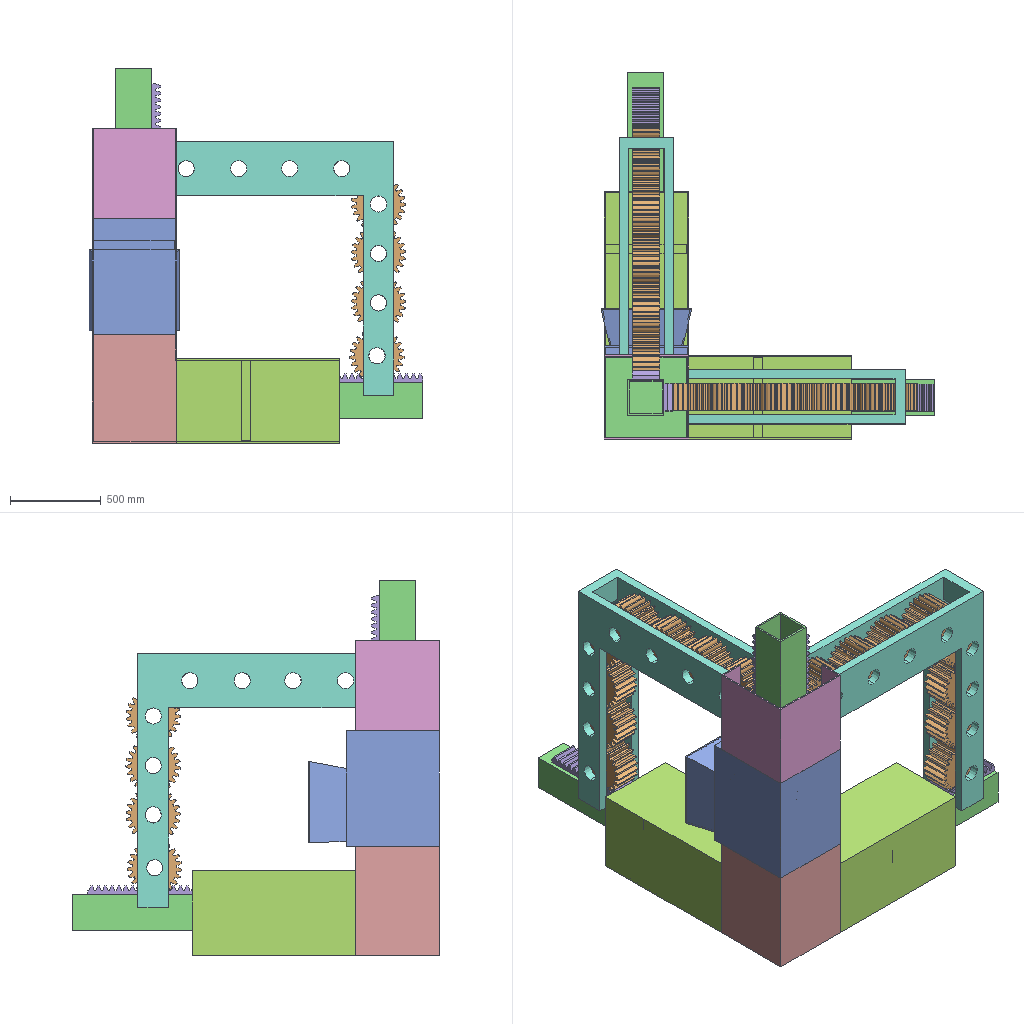Assembly | SolidWorks | 8 different items | 30 placed | box 1844 x 2026 x 2068 mm
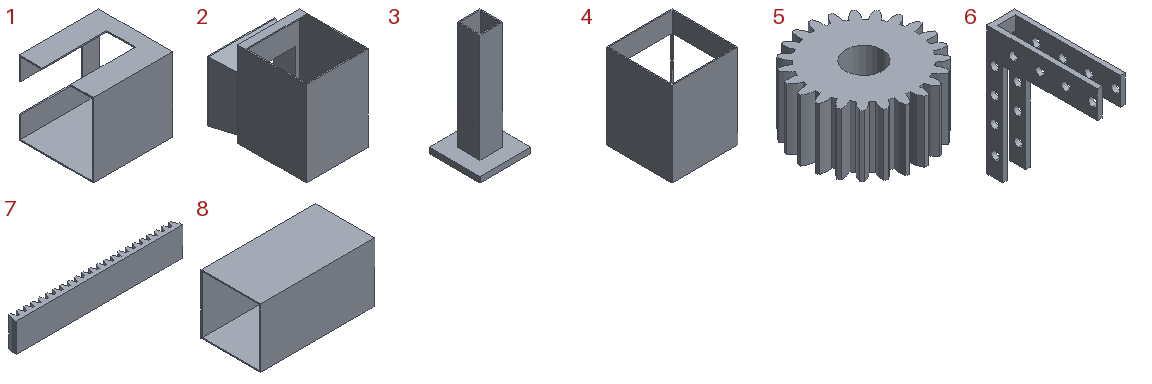Parts list (item | quantity | size | volume | features):
1 | x1 | 500 x 466 x 466 mm | 6178880 mm3 | features Cut 2, DeleteBody 1, Extrusion 1, MoveCopyBody 1, Stock 1
2 | x1 | 500 x 724 x 640 mm | 11993841 mm3 | features ICE 5, Blend 1, Extrusion 1, Shell 1
3 | x3 | 445 x 445 x 1000 mm | 17121250 mm3 | features Extrusion 1, ICE 1
4 | x1 | 466 x 466 x 600 mm | 7173600 mm3 | features ICE 3, Extrusion 1
5 | x16 | 299.728 x 299.348 x 150 mm | 7864200 mm3 | features ICE 2, CirPattern 1, Extrusion 1
6 | x2 | 300 x 1200 x 1400 mm | 51410620 mm3 | features ICE 6, Cut 3, Extrusion 1
7 | x4 | 867.08 x 47 x 150 mm | 4458786 mm3 | features Extrusion 1, ICE 1
8 | x2 | 900 x 466 x 466 mm | 13190400 mm3 | features Extrusion 1
Mates (type | each side: item.copy, entity, surface, feature):
Coincident | 4.1 face plane Boss-Extrude1 | 2.1 face plane Boss-Extrude1 | 3 times
Coincident | 4.1 face plane Boss-Extrude1 | 8.1 face plane Boss-Extrude1 | 3 times
Coincident | 2.1 face plane Boss-Extrude1 | 1.1 face plane Boss-Extrude1 | 3 times
Coincident | 4.1 face plane Boss-Extrude1 | 8.2 face plane Boss-Extrude1 | 3 times
DistanceDim | assembly face | 1.1 face plane Boss-Extrude1 | 2 times
DistanceDim | assembly face | 8.1 face plane Boss-Extrude1
DistanceDim | 8.1 face plane Boss-Extrude1 | assembly face
DistanceDim | assembly face | 8.2 face plane Boss-Extrude1
DistanceDim | 8.2 face plane Boss-Extrude1 | assembly face
DistanceDim | assembly face | 4.1 face plane Boss-Extrude2
DistanceDim | assembly face | 4.1 face plane Boss-Extrude1
DistanceDim | 4.1 face plane Boss-Extrude1 | assembly face
Coincident | 1.1 face plane Boss-Extrude1 | 6.1 face plane Boss-Extrude1
Width | 8.2 face plane Boss-Extrude1 | 8.2 face plane Boss-Extrude1 | 6.1 face plane Boss-Extrude1 | 6.1 face plane Boss-Extrude1
Coincident | 1.1 face plane Boss-Extrude1 | 6.2 face plane Boss-Extrude1
Width | 8.1 face plane Boss-Extrude1 | 8.1 face plane Boss-Extrude1 | 6.2 face plane Boss-Extrude1 | 6.2 face plane Boss-Extrude1
Concentric | 6.1 face cylinder Cut-Extrude2 | 5.1 face cylinder Cut-Extrude1
Width | 6.1 face plane Boss-Extrude1 | 6.1 face plane Boss-Extrude1 | 5.1 face plane Boss-Extrude1 | 5.1 face plane Boss-Extrude1
Parallel | 6.1 face plane Boss-Extrude1 | assembly face | 2 times
Width | 6.1 face plane Boss-Extrude1 | 6.1 face plane Boss-Extrude1 | assembly face | assembly face | 2 times
Coincident | assembly face | 7.1 face plane Boss-Extrude1 | 2 times
Width | assembly face | assembly face | 7.1 face plane Boss-Extrude1 | 7.1 face plane Boss-Extrude1
Concentric | 6.1 face cylinder Cut-Extrude2 | 5.2 face cylinder Cut-Extrude1
Coincident | 5.1 face plane Boss-Extrude1 | 5.2 face plane Boss-Extrude1
Coincident | 8.2 face plane Boss-Extrude1 | assembly face
Coincident | 5.2 face plane Boss-Extrude1 | assembly face
Concentric | 6.1 face cylinder Cut-Extrude2 | 5.3 face cylinder Cut-Extrude1
Concentric | 6.1 face cylinder Cut-Extrude1 | 5.4 face cylinder Cut-Extrude1
Coincident | 5.3 face plane Boss-Extrude1 | 5.4 face plane Boss-Extrude1
Parallel | 5.1 face plane Boss-Extrude1 | 5.3 face plane Boss-Extrude1
Coincident | 5.1 face plane Boss-Extrude1 | 5.3 face plane Boss-Extrude1
GearDim | 5.4 face cylinder Boss-Extrude1 | 5.3 face cylinder CirPattern1
GearDim | 5.1 face cylinder Boss-Extrude2 | 5.3 face cylinder Boss-Extrude1
GearDim | 5.1 face cylinder Boss-Extrude1 | 5.2 face cylinder CirPattern1
Coincident | 5.2 face plane Boss-Extrude1 | 5.5 face plane Boss-Extrude1
Concentric | 6.1 face cylinder Cut-Extrude4 | 5.5 face cylinder Cut-Extrude1
Coincident | 8.2 face plane Boss-Extrude1 | 3.1 face plane Boss-Extrude1 | 2 times
Width | 3.1 face plane Boss-Extrude2 | 3.1 face plane Boss-Extrude2 | 7.1 face plane Boss-Extrude1 | 7.1 face plane Boss-Extrude1
Coincident | 7.1 face plane Boss-Extrude1 | 3.1 face plane Boss-Extrude2
Coincident | 7.1 face plane Boss-Extrude1 | 3.1 face plane Boss-Extrude1
GearDim | 5.5 face cylinder CirPattern1 | 5.2 face cylinder Boss-Extrude1
Concentric | 6.1 face cylinder Cut-Extrude1 | 5.6 face cylinder Cut-Extrude1
Coincident | 5.4 face plane Boss-Extrude1 | 5.6 face plane Boss-Extrude1
Concentric | 6.1 face cylinder Cut-Extrude1 | 5.7 face cylinder Cut-Extrude1
Coincident | 5.6 face plane Boss-Extrude1 | 5.7 face plane Boss-Extrude1
Coincident | assembly face | 7.2 face plane Boss-Extrude1 | 2 times
Width | assembly face | assembly face | 7.2 face plane Boss-Extrude1 | 7.2 face plane Boss-Extrude1
GearDim | 5.4 face cylinder Boss-Extrude1 | 5.6 face cylinder Boss-Extrude2
GearDim | 5.6 face cylinder Boss-Extrude1 | 5.7 face cylinder CirPattern1
Coincident | 2.1 face plane Boss-Extrude1 | 3.2 face plane Boss-Extrude1
Coincident | 1.1 face plane Boss-Extrude1 | 3.2 face plane Boss-Extrude1
Width | 3.2 face plane Boss-Extrude2 | 3.2 face plane Boss-Extrude2 | 7.2 face plane Boss-Extrude1 | 7.2 face plane Boss-Extrude1
Coincident | 7.2 face plane Boss-Extrude1 | 3.2 face plane Boss-Extrude2
Concentric | 6.2 face cylinder Cut-Extrude2 | 5.8 face cylinder Cut-Extrude1
Concentric | 6.2 face cylinder Cut-Extrude2 | assembly face
Concentric | 6.2 face cylinder Cut-Extrude2 | 5.9 face cylinder Cut-Extrude1
Concentric | 6.2 face cylinder Cut-Extrude4 | 5.10 face cylinder Cut-Extrude1
Coincident | 8.1 face plane Boss-Extrude1 | 3.3 face plane Boss-Extrude1 | 2 times
Coincident | 7.3 face plane Boss-Extrude1 | 3.3 face plane Boss-Extrude2 | 2 times
Width | 3.3 face plane Boss-Extrude2 | 3.3 face plane Boss-Extrude2 | 7.3 face plane Boss-Extrude1 | 7.3 face plane Boss-Extrude1
Width | 6.2 face plane Boss-Extrude1 | 6.2 face plane Boss-Extrude1 | 5.10 face plane Boss-Extrude1 | 5.10 face plane Boss-Extrude1
Coincident | 5.9 face plane Boss-Extrude1 | 5.10 face plane Boss-Extrude1
Coincident | assembly face | 5.9 face plane Boss-Extrude1
Coincident | 5.8 face plane Boss-Extrude1 | assembly face
Concentric | 6.2 face cylinder Cut-Extrude1 | 5.11 face cylinder Cut-Extrude1
Concentric | 6.2 edge | 5.12 face cylinder Cut-Extrude1
Concentric | 6.2 face cylinder Cut-Extrude1 | 5.13 face cylinder Cut-Extrude1
Coincident | 5.8 face plane Boss-Extrude1 | 5.13 face plane Boss-Extrude1
Coincident | 5.12 face plane Boss-Extrude1 | 5.13 face plane Boss-Extrude1
Coincident | 5.11 face plane Boss-Extrude1 | 5.12 face plane Boss-Extrude1
Coincident | 3.2 face plane Boss-Extrude2 | assembly face | 2 times
Width | 3.2 face plane Boss-Extrude2 | 3.2 face plane Boss-Extrude2 | assembly face | assembly face
Coincident | 3.2 face plane Boss-Extrude2 | 7.4 face plane Boss-Extrude1
Width | 3.2 face plane Boss-Extrude2 | 3.2 face plane Boss-Extrude2 | 7.4 face plane Boss-Extrude1 | 7.4 face plane Boss-Extrude1
Coincident | 5.9 face plane Boss-Extrude1 | 5.14 face plane Boss-Extrude1
Concentric | 6.2 face cylinder Cut-Extrude2 | 5.14 face cylinder Cut-Extrude1
GearDim | 5.10 face cylinder CirPattern1 | 5.9 face cylinder Boss-Extrude1
GearDim | 5.14 face cylinder Boss-Extrude1 | 5.9 face cylinder CirPattern1
GearDim | 5.14 face cylinder CirPattern1 | 5.8 face cylinder Boss-Extrude1
GearDim | 5.11 face cylinder Boss-Extrude1 | 5.8 face cylinder CirPattern1
GearDim | 5.11 face cylinder CirPattern1 | 5.12 face cylinder Boss-Extrude1
GearDim | 5.13 face cylinder Boss-Extrude1 | 5.12 face cylinder CirPattern1
Concentric | 6.2 face cylinder Cut-Extrude1 | 5.12 face cylinder Cut-Extrude1
Width | 6.2 face plane Boss-Extrude1 | 6.2 face plane Boss-Extrude1 | 5.12 face plane Boss-Extrude1 | 5.12 face plane Boss-Extrude1
Coincident | 5.8 face plane Boss-Extrude1 | 5.15 face plane Boss-Extrude1
Parallel | 5.11 face cylinder Cut-Extrude1 | 5.15 face cylinder Cut-Extrude1
Concentric | 6.2 face cylinder Cut-Extrude5 | 5.15 face cylinder Cut-Extrude1
GearDim | 5.11 face cylinder Boss-Extrude1 | 5.15 face cylinder CirPattern1
Concentric | 6.1 face cylinder Cut-Extrude5 | 5.16 face cylinder Cut-Extrude1
Coincident | 5.4 face plane Boss-Extrude1 | 5.16 face plane Boss-Extrude1
GearDim | 5.4 face cylinder Boss-Extrude1 | 5.16 face cylinder CirPattern1
Coincident | 3.2 face plane Boss-Extrude1 | 7.4 face plane Boss-Extrude2
Coincident | 7.2 face plane Boss-Extrude1 | 7.4 face plane Boss-Extrude1
RackPinionDim | 7.3 select_type:24 | 5.10 select_type:24
RackPinionDim | 7.4 select_type:24 | 5.13 select_type:24
RackPinionDim | 7.2 select_type:24 | 5.7 select_type:24
RackPinionDim | 7.1 select_type:24 | 5.5 select_type:24